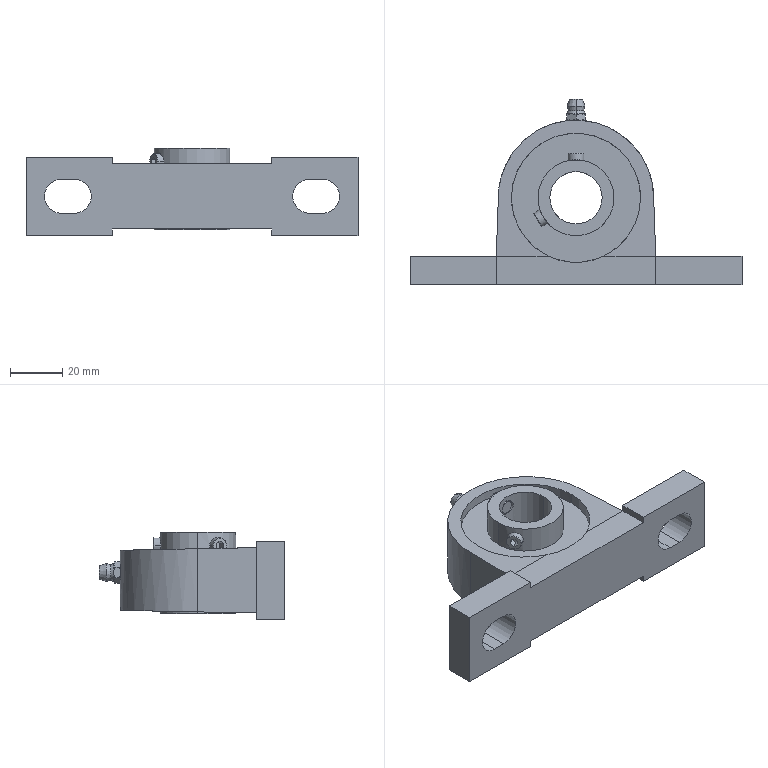Part | STEP file | UCSP204S6-Housing | 1 solid | 105 faces | box 127 x 71.1 x 33.3 mm | volume 85061 mm3 | plane 52 | cylinder 25 | cone 24 | torus 4 | commonest cylinder face diameters 6 x8 13 x4 29.06 x4 49.41 x4 7 x2 20 x2